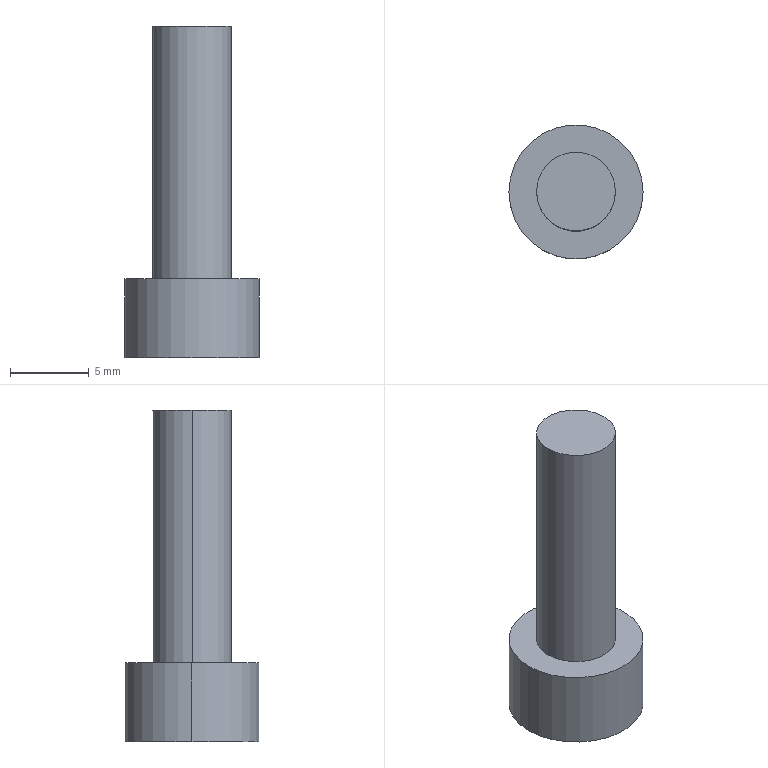Part | STEP file | LG M5_1.6F | 1 solid | 14 faces | box 8.5 x 8.5 x 21 mm | volume 562.896 mm3 | plane 10 | cylinder 4 | commonest cylinder face diameters 5 x2 8.5 x2
STEP:
#1=CARTESIAN_POINT('',(0.,0.,0.));
#2=DIRECTION('',(0.,0.,1.));
#3=DIRECTION('',(1.,0.,0.));
#4=AXIS2_PLACEMENT_3D('',#1,#2,#3);
#5=CARTESIAN_POINT('',(2.5,0.,16.));
#6=VERTEX_POINT('',#5);
#7=CARTESIAN_POINT('',(-2.5,0.,16.));
#8=VERTEX_POINT('',#7);
#9=CARTESIAN_POINT('',(0.,0.,16.));
#10=DIRECTION('',(0.,0.,1.));
#11=DIRECTION('',(1.,0.,0.));
#12=AXIS2_PLACEMENT_3D('',#9,#10,#11);
#13=CIRCLE('',#12,2.5);
#14=CARTESIAN_POINT('',(0.,0.,16.));
#15=DIRECTION('',(0.,0.,-1.));
#16=DIRECTION('',(-1.,0.,0.));
#17=AXIS2_PLACEMENT_3D('',#14,#15,#16);
#18=CYLINDRICAL_SURFACE('',#17,2.5);
#19=CARTESIAN_POINT('',(3.142,0.));
#20=DIRECTION('',(-1.,0.));
#21=VECTOR('',#20,1.);
#22=LINE('',#19,#21);
#23=(GEOMETRIC_REPRESENTATION_CONTEXT(2)PARAMETRIC_REPRESENTATION_CONTEXT()REPRESENTATION_CONTEXT('',''));
#24=DEFINITIONAL_REPRESENTATION('',(#22),#23);
#25=PCURVE('',#18,#24);
#26=CARTESIAN_POINT('',(0.,0.,16.));
#27=DIRECTION('',(0.,0.,1.));
#28=DIRECTION('',(1.,0.,0.));
#29=AXIS2_PLACEMENT_3D('',#26,#27,#28);
#30=PLANE('',#29);
#31=CARTESIAN_POINT('',(0.,0.));
#32=DIRECTION('',(1.,0.));
#33=AXIS2_PLACEMENT_2D('',#31,#32);
#34=CIRCLE('',#33,2.5);
#35=(GEOMETRIC_REPRESENTATION_CONTEXT(2)PARAMETRIC_REPRESENTATION_CONTEXT()REPRESENTATION_CONTEXT('',''));
#36=DEFINITIONAL_REPRESENTATION('',(#34),#35);
#37=PCURVE('',#30,#36);
#38=SURFACE_CURVE('',#13,(#25,#37),.PCURVE_S1.);
#39=EDGE_CURVE('',#6,#8,#38,.T.);
#40=ORIENTED_EDGE('',*,*,#39,.F.);
#41=CARTESIAN_POINT('',(2.5,0.,0.));
#42=VERTEX_POINT('',#41);
#43=CARTESIAN_POINT('',(2.5,0.,16.));
#44=DIRECTION('',(0.,0.,-1.));
#45=VECTOR('',#44,1.);
#46=LINE('',#43,#45);
#47=CARTESIAN_POINT('',(3.142,0.));
#48=DIRECTION('',(0.,1.));
#49=VECTOR('',#48,1.);
#50=LINE('',#47,#49);
#51=(GEOMETRIC_REPRESENTATION_CONTEXT(2)PARAMETRIC_REPRESENTATION_CONTEXT()REPRESENTATION_CONTEXT('',''));
#52=DEFINITIONAL_REPRESENTATION('',(#50),#51);
#53=PCURVE('',#18,#52);
#54=CARTESIAN_POINT('',(0.,0.,16.));
#55=DIRECTION('',(0.,0.,-1.));
#56=DIRECTION('',(-1.,0.,0.));
#57=AXIS2_PLACEMENT_3D('',#54,#55,#56);
#58=CYLINDRICAL_SURFACE('',#57,2.5);
#59=CARTESIAN_POINT('',(3.142,0.));
#60=DIRECTION('',(0.,1.));
#61=VECTOR('',#60,1.);
#62=LINE('',#59,#61);
#63=(GEOMETRIC_REPRESENTATION_CONTEXT(2)PARAMETRIC_REPRESENTATION_CONTEXT()REPRESENTATION_CONTEXT('',''));
#64=DEFINITIONAL_REPRESENTATION('',(#62),#63);
#65=PCURVE('',#58,#64);
#66=SURFACE_CURVE('',#46,(#53,#65),.PCURVE_S1.);
#67=EDGE_CURVE('',#6,#42,#66,.T.);
#68=ORIENTED_EDGE('',*,*,#67,.T.);
#69=CARTESIAN_POINT('',(-2.5,0.,0.));
#70=VERTEX_POINT('',#69);
#71=CARTESIAN_POINT('',(0.,0.,0.));
#72=DIRECTION('',(0.,0.,1.));
#73=DIRECTION('',(1.,0.,0.));
#74=AXIS2_PLACEMENT_3D('',#71,#72,#73);
#75=CIRCLE('',#74,2.5);
#76=CARTESIAN_POINT('',(3.142,16.));
#77=DIRECTION('',(-1.,0.));
#78=VECTOR('',#77,1.);
#79=LINE('',#76,#78);
#80=(GEOMETRIC_REPRESENTATION_CONTEXT(2)PARAMETRIC_REPRESENTATION_CONTEXT()REPRESENTATION_CONTEXT('',''));
#81=DEFINITIONAL_REPRESENTATION('',(#79),#80);
#82=PCURVE('',#18,#81);
#83=CARTESIAN_POINT('',(0.,0.,0.));
#84=DIRECTION('',(0.,0.,1.));
#85=DIRECTION('',(1.,0.,0.));
#86=AXIS2_PLACEMENT_3D('',#83,#84,#85);
#87=PLANE('',#86);
#88=CARTESIAN_POINT('',(0.,0.));
#89=DIRECTION('',(1.,0.));
#90=AXIS2_PLACEMENT_2D('',#88,#89);
#91=CIRCLE('',#90,2.5);
#92=(GEOMETRIC_REPRESENTATION_CONTEXT(2)PARAMETRIC_REPRESENTATION_CONTEXT()REPRESENTATION_CONTEXT('',''));
#93=DEFINITIONAL_REPRESENTATION('',(#91),#92);
#94=PCURVE('',#87,#93);
#95=SURFACE_CURVE('',#75,(#82,#94),.PCURVE_S1.);
#96=EDGE_CURVE('',#42,#70,#95,.T.);
#97=ORIENTED_EDGE('',*,*,#96,.T.);
#98=CARTESIAN_POINT('',(-2.5,0.,16.));
#99=DIRECTION('',(0.,0.,-1.));
#100=VECTOR('',#99,1.);
#101=LINE('',#98,#100);
#102=CARTESIAN_POINT('',(0.,0.));
#103=DIRECTION('',(0.,1.));
#104=VECTOR('',#103,1.);
#105=LINE('',#102,#104);
#106=(GEOMETRIC_REPRESENTATION_CONTEXT(2)PARAMETRIC_REPRESENTATION_CONTEXT()REPRESENTATION_CONTEXT('',''));
#107=DEFINITIONAL_REPRESENTATION('',(#105),#106);
#108=PCURVE('',#18,#107);
#109=CARTESIAN_POINT('',(6.283,0.));
#110=DIRECTION('',(0.,1.));
#111=VECTOR('',#110,1.);
#112=LINE('',#109,#111);
#113=(GEOMETRIC_REPRESENTATION_CONTEXT(2)PARAMETRIC_REPRESENTATION_CONTEXT()REPRESENTATION_CONTEXT('',''));
#114=DEFINITIONAL_REPRESENTATION('',(#112),#113);
#115=PCURVE('',#58,#114);
#116=SURFACE_CURVE('',#101,(#108,#115),.PCURVE_S1.);
#117=EDGE_CURVE('',#8,#70,#116,.T.);
#118=ORIENTED_EDGE('',*,*,#117,.F.);
#119=EDGE_LOOP('',(#40,#68,#97,#118));
#120=FACE_BOUND('',#119,.T.);
#121=ADVANCED_FACE('',(#120),#18,.T.);
#122=CARTESIAN_POINT('',(4.25,0.,-5.));
#123=VERTEX_POINT('',#122);
#124=CARTESIAN_POINT('',(-4.25,0.,-5.));
#125=VERTEX_POINT('',#124);
#126=CARTESIAN_POINT('',(0.,0.,-5.));
#127=DIRECTION('',(0.,0.,1.));
#128=DIRECTION('',(1.,0.,0.));
#129=AXIS2_PLACEMENT_3D('',#126,#127,#128);
#130=CIRCLE('',#129,4.25);
#131=CARTESIAN_POINT('',(0.,0.,-5.));
#132=DIRECTION('',(0.,0.,1.));
#133=DIRECTION('',(1.,0.,0.));
#134=AXIS2_PLACEMENT_3D('',#131,#132,#133);
#135=CYLINDRICAL_SURFACE('',#134,4.25);
#136=CARTESIAN_POINT('',(0.,0.));
#137=DIRECTION('',(1.,0.));
#138=VECTOR('',#137,1.);
#139=LINE('',#136,#138);
#140=(GEOMETRIC_REPRESENTATION_CONTEXT(2)PARAMETRIC_REPRESENTATION_CONTEXT()REPRESENTATION_CONTEXT('',''));
#141=DEFINITIONAL_REPRESENTATION('',(#139),#140);
#142=PCURVE('',#135,#141);
#143=CARTESIAN_POINT('',(0.,0.,-5.));
#144=DIRECTION('',(0.,0.,1.));
#145=DIRECTION('',(1.,0.,0.));
#146=AXIS2_PLACEMENT_3D('',#143,#144,#145);
#147=PLANE('',#146);
#148=CARTESIAN_POINT('',(0.,0.));
#149=DIRECTION('',(1.,0.));
#150=AXIS2_PLACEMENT_2D('',#148,#149);
#151=CIRCLE('',#150,4.25);
#152=(GEOMETRIC_REPRESENTATION_CONTEXT(2)PARAMETRIC_REPRESENTATION_CONTEXT()REPRESENTATION_CONTEXT('',''));
#153=DEFINITIONAL_REPRESENTATION('',(#151),#152);
#154=PCURVE('',#147,#153);
#155=SURFACE_CURVE('',#130,(#142,#154),.PCURVE_S1.);
#156=EDGE_CURVE('',#123,#125,#155,.T.);
#157=ORIENTED_EDGE('',*,*,#156,.T.);
#158=CARTESIAN_POINT('',(-4.25,0.,0.));
#159=VERTEX_POINT('',#158);
#160=CARTESIAN_POINT('',(-4.25,0.,-5.));
#161=DIRECTION('',(0.,0.,1.));
#162=VECTOR('',#161,1.);
#163=LINE('',#160,#162);
#164=CARTESIAN_POINT('',(3.142,0.));
#165=DIRECTION('',(0.,1.));
#166=VECTOR('',#165,1.);
#167=LINE('',#164,#166);
#168=(GEOMETRIC_REPRESENTATION_CONTEXT(2)PARAMETRIC_REPRESENTATION_CONTEXT()REPRESENTATION_CONTEXT('',''));
#169=DEFINITIONAL_REPRESENTATION('',(#167),#168);
#170=PCURVE('',#135,#169);
#171=CARTESIAN_POINT('',(0.,0.,-5.));
#172=DIRECTION('',(0.,0.,1.));
#173=DIRECTION('',(1.,0.,0.));
#174=AXIS2_PLACEMENT_3D('',#171,#172,#173);
#175=CYLINDRICAL_SURFACE('',#174,4.25);
#176=CARTESIAN_POINT('',(3.142,0.));
#177=DIRECTION('',(0.,1.));
#178=VECTOR('',#177,1.);
#179=LINE('',#176,#178);
#180=(GEOMETRIC_REPRESENTATION_CONTEXT(2)PARAMETRIC_REPRESENTATION_CONTEXT()REPRESENTATION_CONTEXT('',''));
#181=DEFINITIONAL_REPRESENTATION('',(#179),#180);
#182=PCURVE('',#175,#181);
#183=SURFACE_CURVE('',#163,(#170,#182),.PCURVE_S1.);
#184=EDGE_CURVE('',#125,#159,#183,.T.);
#185=ORIENTED_EDGE('',*,*,#184,.T.);
#186=CARTESIAN_POINT('',(4.25,0.,0.));
#187=VERTEX_POINT('',#186);
#188=CARTESIAN_POINT('',(0.,0.,0.));
#189=DIRECTION('',(0.,0.,1.));
#190=DIRECTION('',(1.,0.,0.));
#191=AXIS2_PLACEMENT_3D('',#188,#189,#190);
#192=CIRCLE('',#191,4.25);
#193=CARTESIAN_POINT('',(0.,5.));
#194=DIRECTION('',(1.,0.));
#195=VECTOR('',#194,1.);
#196=LINE('',#193,#195);
#197=(GEOMETRIC_REPRESENTATION_CONTEXT(2)PARAMETRIC_REPRESENTATION_CONTEXT()REPRESENTATION_CONTEXT('',''));
#198=DEFINITIONAL_REPRESENTATION('',(#196),#197);
#199=PCURVE('',#135,#198);
#200=CARTESIAN_POINT('',(0.,0.));
#201=DIRECTION('',(1.,0.));
#202=AXIS2_PLACEMENT_2D('',#200,#201);
#203=CIRCLE('',#202,4.25);
#204=(GEOMETRIC_REPRESENTATION_CONTEXT(2)PARAMETRIC_REPRESENTATION_CONTEXT()REPRESENTATION_CONTEXT('',''));
#205=DEFINITIONAL_REPRESENTATION('',(#203),#204);
#206=PCURVE('',#87,#205);
#207=SURFACE_CURVE('',#192,(#199,#206),.PCURVE_S1.);
#208=EDGE_CURVE('',#187,#159,#207,.T.);
#209=ORIENTED_EDGE('',*,*,#208,.F.);
#210=CARTESIAN_POINT('',(4.25,0.,-5.));
#211=DIRECTION('',(0.,0.,1.));
#212=VECTOR('',#211,1.);
#213=LINE('',#210,#212);
#214=CARTESIAN_POINT('',(0.,0.));
#215=DIRECTION('',(0.,1.));
#216=VECTOR('',#215,1.);
#217=LINE('',#214,#216);
#218=(GEOMETRIC_REPRESENTATION_CONTEXT(2)PARAMETRIC_REPRESENTATION_CONTEXT()REPRESENTATION_CONTEXT('',''));
#219=DEFINITIONAL_REPRESENTATION('',(#217),#218);
#220=PCURVE('',#135,#219);
#221=CARTESIAN_POINT('',(6.283,0.));
#222=DIRECTION('',(0.,1.));
#223=VECTOR('',#222,1.);
#224=LINE('',#221,#223);
#225=(GEOMETRIC_REPRESENTATION_CONTEXT(2)PARAMETRIC_REPRESENTATION_CONTEXT()REPRESENTATION_CONTEXT('',''));
#226=DEFINITIONAL_REPRESENTATION('',(#224),#225);
#227=PCURVE('',#175,#226);
#228=SURFACE_CURVE('',#213,(#220,#227),.PCURVE_S1.);
#229=EDGE_CURVE('',#123,#187,#228,.T.);
#230=ORIENTED_EDGE('',*,*,#229,.F.);
#231=EDGE_LOOP('',(#157,#185,#209,#230));
#232=FACE_BOUND('',#231,.T.);
#233=ADVANCED_FACE('',(#232),#135,.T.);
#234=ORIENTED_EDGE('',*,*,#208,.T.);
#235=CARTESIAN_POINT('',(0.,0.,0.));
#236=DIRECTION('',(0.,0.,1.));
#237=DIRECTION('',(1.,0.,0.));
#238=AXIS2_PLACEMENT_3D('',#235,#236,#237);
#239=CIRCLE('',#238,4.25);
#240=CARTESIAN_POINT('',(0.,0.));
#241=DIRECTION('',(1.,0.));
#242=AXIS2_PLACEMENT_2D('',#240,#241);
#243=CIRCLE('',#242,4.25);
#244=(GEOMETRIC_REPRESENTATION_CONTEXT(2)PARAMETRIC_REPRESENTATION_CONTEXT()REPRESENTATION_CONTEXT('',''));
#245=DEFINITIONAL_REPRESENTATION('',(#243),#244);
#246=PCURVE('',#87,#245);
#247=CARTESIAN_POINT('',(0.,5.));
#248=DIRECTION('',(1.,0.));
#249=VECTOR('',#248,1.);
#250=LINE('',#247,#249);
#251=(GEOMETRIC_REPRESENTATION_CONTEXT(2)PARAMETRIC_REPRESENTATION_CONTEXT()REPRESENTATION_CONTEXT('',''));
#252=DEFINITIONAL_REPRESENTATION('',(#250),#251);
#253=PCURVE('',#175,#252);
#254=SURFACE_CURVE('',#239,(#246,#253),.PCURVE_S1.);
#255=EDGE_CURVE('',#159,#187,#254,.T.);
#256=ORIENTED_EDGE('',*,*,#255,.T.);
#257=EDGE_LOOP('',(#234,#256));
#258=FACE_BOUND('',#257,.T.);
#259=CARTESIAN_POINT('',(0.,0.,0.));
#260=DIRECTION('',(0.,0.,1.));
#261=DIRECTION('',(1.,0.,0.));
#262=AXIS2_PLACEMENT_3D('',#259,#260,#261);
#263=CIRCLE('',#262,2.5);
#264=CARTESIAN_POINT('',(0.,0.));
#265=DIRECTION('',(1.,0.));
#266=AXIS2_PLACEMENT_2D('',#264,#265);
#267=CIRCLE('',#266,2.5);
#268=(GEOMETRIC_REPRESENTATION_CONTEXT(2)PARAMETRIC_REPRESENTATION_CONTEXT()REPRESENTATION_CONTEXT('',''));
#269=DEFINITIONAL_REPRESENTATION('',(#267),#268);
#270=PCURVE('',#87,#269);
#271=CARTESIAN_POINT('',(9.425,16.));
#272=DIRECTION('',(-1.,0.));
#273=VECTOR('',#272,1.);
#274=LINE('',#271,#273);
#275=(GEOMETRIC_REPRESENTATION_CONTEXT(2)PARAMETRIC_REPRESENTATION_CONTEXT()REPRESENTATION_CONTEXT('',''));
#276=DEFINITIONAL_REPRESENTATION('',(#274),#275);
#277=PCURVE('',#58,#276);
#278=SURFACE_CURVE('',#263,(#270,#277),.PCURVE_S1.);
#279=EDGE_CURVE('',#70,#42,#278,.T.);
#280=ORIENTED_EDGE('',*,*,#279,.F.);
#281=ORIENTED_EDGE('',*,*,#96,.F.);
#282=EDGE_LOOP('',(#280,#281));
#283=FACE_BOUND('',#282,.T.);
#284=ADVANCED_FACE('',(#258,#283),#87,.T.);
#285=ORIENTED_EDGE('',*,*,#184,.F.);
#286=CARTESIAN_POINT('',(0.,0.,-5.));
#287=DIRECTION('',(0.,0.,1.));
#288=DIRECTION('',(1.,0.,0.));
#289=AXIS2_PLACEMENT_3D('',#286,#287,#288);
#290=CIRCLE('',#289,4.25);
#291=CARTESIAN_POINT('',(0.,0.));
#292=DIRECTION('',(1.,0.));
#293=VECTOR('',#292,1.);
#294=LINE('',#291,#293);
#295=(GEOMETRIC_REPRESENTATION_CONTEXT(2)PARAMETRIC_REPRESENTATION_CONTEXT()REPRESENTATION_CONTEXT('',''));
#296=DEFINITIONAL_REPRESENTATION('',(#294),#295);
#297=PCURVE('',#175,#296);
#298=CARTESIAN_POINT('',(0.,0.));
#299=DIRECTION('',(1.,0.));
#300=AXIS2_PLACEMENT_2D('',#298,#299);
#301=CIRCLE('',#300,4.25);
#302=(GEOMETRIC_REPRESENTATION_CONTEXT(2)PARAMETRIC_REPRESENTATION_CONTEXT()REPRESENTATION_CONTEXT('',''));
#303=DEFINITIONAL_REPRESENTATION('',(#301),#302);
#304=PCURVE('',#147,#303);
#305=SURFACE_CURVE('',#290,(#297,#304),.PCURVE_S1.);
#306=EDGE_CURVE('',#125,#123,#305,.T.);
#307=ORIENTED_EDGE('',*,*,#306,.T.);
#308=ORIENTED_EDGE('',*,*,#229,.T.);
#309=ORIENTED_EDGE('',*,*,#255,.F.);
#310=EDGE_LOOP('',(#285,#307,#308,#309));
#311=FACE_BOUND('',#310,.T.);
#312=ADVANCED_FACE('',(#311),#175,.T.);
#313=CARTESIAN_POINT('',(-2.321,0.,-5.));
#314=VERTEX_POINT('',#313);
#315=CARTESIAN_POINT('',(-1.16,2.01,-5.));
#316=VERTEX_POINT('',#315);
#317=CARTESIAN_POINT('',(-2.321,0.,-5.));
#318=DIRECTION('',(0.5,0.866,0.));
#319=VECTOR('',#318,1.);
#320=LINE('',#317,#319);
#321=CARTESIAN_POINT('',(-2.321,0.));
#322=DIRECTION('',(0.5,0.866));
#323=VECTOR('',#322,1.);
#324=LINE('',#321,#323);
#325=(GEOMETRIC_REPRESENTATION_CONTEXT(2)PARAMETRIC_REPRESENTATION_CONTEXT()REPRESENTATION_CONTEXT('',''));
#326=DEFINITIONAL_REPRESENTATION('',(#324),#325);
#327=PCURVE('',#147,#326);
#328=CARTESIAN_POINT('',(-2.321,0.,-2.5));
#329=DIRECTION('',(-0.866,0.5,0.));
#330=DIRECTION('',(-0.5,-0.866,0.));
#331=AXIS2_PLACEMENT_3D('',#328,#329,#330);
#332=PLANE('',#331);
#333=CARTESIAN_POINT('',(0.,-2.5));
#334=DIRECTION('',(-1.,0.));
#335=VECTOR('',#334,1.);
#336=LINE('',#333,#335);
#337=(GEOMETRIC_REPRESENTATION_CONTEXT(2)PARAMETRIC_REPRESENTATION_CONTEXT()REPRESENTATION_CONTEXT('',''));
#338=DEFINITIONAL_REPRESENTATION('',(#336),#337);
#339=PCURVE('',#332,#338);
#340=SURFACE_CURVE('',#320,(#327,#339),.PCURVE_S1.);
#341=EDGE_CURVE('',#314,#316,#340,.T.);
#342=ORIENTED_EDGE('',*,*,#341,.F.);
#343=CARTESIAN_POINT('',(-1.16,-2.01,-5.));
#344=VERTEX_POINT('',#343);
#345=CARTESIAN_POINT('',(-1.16,-2.01,-5.));
#346=DIRECTION('',(-0.5,0.866,0.));
#347=VECTOR('',#346,1.);
#348=LINE('',#345,#347);
#349=CARTESIAN_POINT('',(-1.16,-2.01));
#350=DIRECTION('',(-0.5,0.866));
#351=VECTOR('',#350,1.);
#352=LINE('',#349,#351);
#353=(GEOMETRIC_REPRESENTATION_CONTEXT(2)PARAMETRIC_REPRESENTATION_CONTEXT()REPRESENTATION_CONTEXT('',''));
#354=DEFINITIONAL_REPRESENTATION('',(#352),#353);
#355=PCURVE('',#147,#354);
#356=CARTESIAN_POINT('',(-1.16,-2.01,-2.5));
#357=DIRECTION('',(-0.866,-0.5,0.));
#358=DIRECTION('',(0.5,-0.866,0.));
#359=AXIS2_PLACEMENT_3D('',#356,#357,#358);
#360=PLANE('',#359);
#361=CARTESIAN_POINT('',(0.,-2.5));
#362=DIRECTION('',(-1.,0.));
#363=VECTOR('',#362,1.);
#364=LINE('',#361,#363);
#365=(GEOMETRIC_REPRESENTATION_CONTEXT(2)PARAMETRIC_REPRESENTATION_CONTEXT()REPRESENTATION_CONTEXT('',''));
#366=DEFINITIONAL_REPRESENTATION('',(#364),#365);
#367=PCURVE('',#360,#366);
#368=SURFACE_CURVE('',#348,(#355,#367),.PCURVE_S1.);
#369=EDGE_CURVE('',#344,#314,#368,.T.);
#370=ORIENTED_EDGE('',*,*,#369,.F.);
#371=CARTESIAN_POINT('',(1.16,-2.01,-5.));
#372=VERTEX_POINT('',#371);
#373=CARTESIAN_POINT('',(1.16,-2.01,-5.));
#374=DIRECTION('',(-1.,0.,0.));
#375=VECTOR('',#374,1.);
#376=LINE('',#373,#375);
#377=CARTESIAN_POINT('',(1.16,-2.01));
#378=DIRECTION('',(-1.,0.));
#379=VECTOR('',#378,1.);
#380=LINE('',#377,#379);
#381=(GEOMETRIC_REPRESENTATION_CONTEXT(2)PARAMETRIC_REPRESENTATION_CONTEXT()REPRESENTATION_CONTEXT('',''));
#382=DEFINITIONAL_REPRESENTATION('',(#380),#381);
#383=PCURVE('',#147,#382);
#384=CARTESIAN_POINT('',(1.16,-2.01,-2.5));
#385=DIRECTION('',(0.,-1.,0.));
#386=DIRECTION('',(0.,0.,-1.));
#387=AXIS2_PLACEMENT_3D('',#384,#385,#386);
#388=PLANE('',#387);
#389=CARTESIAN_POINT('',(2.5,0.));
#390=DIRECTION('',(0.,-1.));
#391=VECTOR('',#390,1.);
#392=LINE('',#389,#391);
#393=(GEOMETRIC_REPRESENTATION_CONTEXT(2)PARAMETRIC_REPRESENTATION_CONTEXT()REPRESENTATION_CONTEXT('',''));
#394=DEFINITIONAL_REPRESENTATION('',(#392),#393);
#395=PCURVE('',#388,#394);
#396=SURFACE_CURVE('',#376,(#383,#395),.PCURVE_S1.);
#397=EDGE_CURVE('',#372,#344,#396,.T.);
#398=ORIENTED_EDGE('',*,*,#397,.F.);
#399=CARTESIAN_POINT('',(2.321,0.,-5.));
#400=VERTEX_POINT('',#399);
#401=CARTESIAN_POINT('',(2.321,0.,-5.));
#402=DIRECTION('',(-0.5,-0.866,0.));
#403=VECTOR('',#402,1.);
#404=LINE('',#401,#403);
#405=CARTESIAN_POINT('',(2.321,0.));
#406=DIRECTION('',(-0.5,-0.866));
#407=VECTOR('',#406,1.);
#408=LINE('',#405,#407);
#409=(GEOMETRIC_REPRESENTATION_CONTEXT(2)PARAMETRIC_REPRESENTATION_CONTEXT()REPRESENTATION_CONTEXT('',''));
#410=DEFINITIONAL_REPRESENTATION('',(#408),#409);
#411=PCURVE('',#147,#410);
#412=CARTESIAN_POINT('',(2.321,0.,-2.5));
#413=DIRECTION('',(0.866,-0.5,0.));
#414=DIRECTION('',(0.5,0.866,0.));
#415=AXIS2_PLACEMENT_3D('',#412,#413,#414);
#416=PLANE('',#415);
#417=CARTESIAN_POINT('',(0.,-2.5));
#418=DIRECTION('',(-1.,0.));
#419=VECTOR('',#418,1.);
#420=LINE('',#417,#419);
#421=(GEOMETRIC_REPRESENTATION_CONTEXT(2)PARAMETRIC_REPRESENTATION_CONTEXT()REPRESENTATION_CONTEXT('',''));
#422=DEFINITIONAL_REPRESENTATION('',(#420),#421);
#423=PCURVE('',#416,#422);
#424=SURFACE_CURVE('',#404,(#411,#423),.PCURVE_S1.);
#425=EDGE_CURVE('',#400,#372,#424,.T.);
#426=ORIENTED_EDGE('',*,*,#425,.F.);
#427=CARTESIAN_POINT('',(1.16,2.01,-5.));
#428=VERTEX_POINT('',#427);
#429=CARTESIAN_POINT('',(1.16,2.01,-5.));
#430=DIRECTION('',(0.5,-0.866,0.));
#431=VECTOR('',#430,1.);
#432=LINE('',#429,#431);
#433=CARTESIAN_POINT('',(1.16,2.01));
#434=DIRECTION('',(0.5,-0.866));
#435=VECTOR('',#434,1.);
#436=LINE('',#433,#435);
#437=(GEOMETRIC_REPRESENTATION_CONTEXT(2)PARAMETRIC_REPRESENTATION_CONTEXT()REPRESENTATION_CONTEXT('',''));
#438=DEFINITIONAL_REPRESENTATION('',(#436),#437);
#439=PCURVE('',#147,#438);
#440=CARTESIAN_POINT('',(1.16,2.01,-2.5));
#441=DIRECTION('',(0.866,0.5,0.));
#442=DIRECTION('',(-0.5,0.866,0.));
#443=AXIS2_PLACEMENT_3D('',#440,#441,#442);
#444=PLANE('',#443);
#445=CARTESIAN_POINT('',(0.,-2.5));
#446=DIRECTION('',(-1.,0.));
#447=VECTOR('',#446,1.);
#448=LINE('',#445,#447);
#449=(GEOMETRIC_REPRESENTATION_CONTEXT(2)PARAMETRIC_REPRESENTATION_CONTEXT()REPRESENTATION_CONTEXT('',''));
#450=DEFINITIONAL_REPRESENTATION('',(#448),#449);
#451=PCURVE('',#444,#450);
#452=SURFACE_CURVE('',#432,(#439,#451),.PCURVE_S1.);
#453=EDGE_CURVE('',#428,#400,#452,.T.);
#454=ORIENTED_EDGE('',*,*,#453,.F.);
#455=CARTESIAN_POINT('',(-1.16,2.01,-5.));
#456=DIRECTION('',(1.,0.,0.));
#457=VECTOR('',#456,1.);
#458=LINE('',#455,#457);
#459=CARTESIAN_POINT('',(-1.16,2.01));
#460=DIRECTION('',(1.,0.));
#461=VECTOR('',#460,1.);
#462=LINE('',#459,#461);
#463=(GEOMETRIC_REPRESENTATION_CONTEXT(2)PARAMETRIC_REPRESENTATION_CONTEXT()REPRESENTATION_CONTEXT('',''));
#464=DEFINITIONAL_REPRESENTATION('',(#462),#463);
#465=PCURVE('',#147,#464);
#466=CARTESIAN_POINT('',(-1.16,2.01,-2.5));
#467=DIRECTION('',(0.,1.,0.));
#468=DIRECTION('',(0.,0.,1.));
#469=AXIS2_PLACEMENT_3D('',#466,#467,#468);
#470=PLANE('',#469);
#471=CARTESIAN_POINT('',(-2.5,0.));
#472=DIRECTION('',(0.,1.));
#473=VECTOR('',#472,1.);
#474=LINE('',#471,#473);
#475=(GEOMETRIC_REPRESENTATION_CONTEXT(2)PARAMETRIC_REPRESENTATION_CONTEXT()REPRESENTATION_CONTEXT('',''));
#476=DEFINITIONAL_REPRESENTATION('',(#474),#475);
#477=PCURVE('',#470,#476);
#478=SURFACE_CURVE('',#458,(#465,#477),.PCURVE_S1.);
#479=EDGE_CURVE('',#316,#428,#478,.T.);
#480=ORIENTED_EDGE('',*,*,#479,.F.);
#481=EDGE_LOOP('',(#342,#370,#398,#426,#454,#480));
#482=FACE_BOUND('',#481,.T.);
#483=ORIENTED_EDGE('',*,*,#156,.F.);
#484=ORIENTED_EDGE('',*,*,#306,.F.);
#485=EDGE_LOOP('',(#483,#484));
#486=FACE_BOUND('',#485,.T.);
#487=ADVANCED_FACE('',(#482,#486),#147,.F.);
#488=ORIENTED_EDGE('',*,*,#67,.F.);
#489=CARTESIAN_POINT('',(0.,0.,16.));
#490=DIRECTION('',(0.,0.,1.));
#491=DIRECTION('',(1.,0.,0.));
#492=AXIS2_PLACEMENT_3D('',#489,#490,#491);
#493=CIRCLE('',#492,2.5);
#494=CARTESIAN_POINT('',(9.425,0.));
#495=DIRECTION('',(-1.,0.));
#496=VECTOR('',#495,1.);
#497=LINE('',#494,#496);
#498=(GEOMETRIC_REPRESENTATION_CONTEXT(2)PARAMETRIC_REPRESENTATION_CONTEXT()REPRESENTATION_CONTEXT('',''));
#499=DEFINITIONAL_REPRESENTATION('',(#497),#498);
#500=PCURVE('',#58,#499);
#501=CARTESIAN_POINT('',(0.,0.));
#502=DIRECTION('',(1.,0.));
#503=AXIS2_PLACEMENT_2D('',#501,#502);
#504=CIRCLE('',#503,2.5);
#505=(GEOMETRIC_REPRESENTATION_CONTEXT(2)PARAMETRIC_REPRESENTATION_CONTEXT()REPRESENTATION_CONTEXT('',''));
#506=DEFINITIONAL_REPRESENTATION('',(#504),#505);
#507=PCURVE('',#30,#506);
#508=SURFACE_CURVE('',#493,(#500,#507),.PCURVE_S1.);
#509=EDGE_CURVE('',#8,#6,#508,.T.);
#510=ORIENTED_EDGE('',*,*,#509,.F.);
#511=ORIENTED_EDGE('',*,*,#117,.T.);
#512=ORIENTED_EDGE('',*,*,#279,.T.);
#513=EDGE_LOOP('',(#488,#510,#511,#512));
#514=FACE_BOUND('',#513,.T.);
#515=ADVANCED_FACE('',(#514),#58,.T.);
#516=ORIENTED_EDGE('',*,*,#509,.T.);
#517=ORIENTED_EDGE('',*,*,#39,.T.);
#518=EDGE_LOOP('',(#516,#517));
#519=FACE_BOUND('',#518,.T.);
#520=ADVANCED_FACE('',(#519),#30,.T.);
#521=ORIENTED_EDGE('',*,*,#369,.T.);
#522=CARTESIAN_POINT('',(-2.321,0.,-2.5));
#523=VERTEX_POINT('',#522);
#524=CARTESIAN_POINT('',(-2.321,0.,-2.5));
#525=DIRECTION('',(0.,0.,-1.));
#526=VECTOR('',#525,1.);
#527=LINE('',#524,#526);
#528=CARTESIAN_POINT('',(-2.321,0.));
#529=DIRECTION('',(0.,-1.));
#530=VECTOR('',#529,1.);
#531=LINE('',#528,#530);
#532=(GEOMETRIC_REPRESENTATION_CONTEXT(2)PARAMETRIC_REPRESENTATION_CONTEXT()REPRESENTATION_CONTEXT('',''));
#533=DEFINITIONAL_REPRESENTATION('',(#531),#532);
#534=PCURVE('',#360,#533);
#535=CARTESIAN_POINT('',(0.,0.));
#536=DIRECTION('',(0.,-1.));
#537=VECTOR('',#536,1.);
#538=LINE('',#535,#537);
#539=(GEOMETRIC_REPRESENTATION_CONTEXT(2)PARAMETRIC_REPRESENTATION_CONTEXT()REPRESENTATION_CONTEXT('',''));
#540=DEFINITIONAL_REPRESENTATION('',(#538),#539);
#541=PCURVE('',#332,#540);
#542=SURFACE_CURVE('',#527,(#534,#541),.PCURVE_S1.);
#543=EDGE_CURVE('',#523,#314,#542,.T.);
#544=ORIENTED_EDGE('',*,*,#543,.F.);
#545=CARTESIAN_POINT('',(-1.16,-2.01,-2.5));
#546=VERTEX_POINT('',#545);
#547=CARTESIAN_POINT('',(-1.16,-2.01,-2.5));
#548=DIRECTION('',(-0.5,0.866,0.));
#549=VECTOR('',#548,1.);
#550=LINE('',#547,#549);
#551=CARTESIAN_POINT('',(0.,0.));
#552=DIRECTION('',(-1.,0.));
#553=VECTOR('',#552,1.);
#554=LINE('',#551,#553);
#555=(GEOMETRIC_REPRESENTATION_CONTEXT(2)PARAMETRIC_REPRESENTATION_CONTEXT()REPRESENTATION_CONTEXT('',''));
#556=DEFINITIONAL_REPRESENTATION('',(#554),#555);
#557=PCURVE('',#360,#556);
#558=CARTESIAN_POINT('',(0.,0.,-2.5));
#559=DIRECTION('',(0.,0.,-1.));
#560=DIRECTION('',(-1.,0.,0.));
#561=AXIS2_PLACEMENT_3D('',#558,#559,#560);
#562=PLANE('',#561);
#563=CARTESIAN_POINT('',(1.16,-2.01));
#564=DIRECTION('',(0.5,0.866));
#565=VECTOR('',#564,1.);
#566=LINE('',#563,#565);
#567=(GEOMETRIC_REPRESENTATION_CONTEXT(2)PARAMETRIC_REPRESENTATION_CONTEXT()REPRESENTATION_CONTEXT('',''));
#568=DEFINITIONAL_REPRESENTATION('',(#566),#567);
#569=PCURVE('',#562,#568);
#570=SURFACE_CURVE('',#550,(#557,#569),.PCURVE_S1.);
#571=EDGE_CURVE('',#546,#523,#570,.T.);
#572=ORIENTED_EDGE('',*,*,#571,.F.);
#573=CARTESIAN_POINT('',(-1.16,-2.01,-2.5));
#574=DIRECTION('',(0.,0.,-1.));
#575=VECTOR('',#574,1.);
#576=LINE('',#573,#575);
#577=CARTESIAN_POINT('',(0.,0.));
#578=DIRECTION('',(0.,-1.));
#579=VECTOR('',#578,1.);
#580=LINE('',#577,#579);
#581=(GEOMETRIC_REPRESENTATION_CONTEXT(2)PARAMETRIC_REPRESENTATION_CONTEXT()REPRESENTATION_CONTEXT('',''));
#582=DEFINITIONAL_REPRESENTATION('',(#580),#581);
#583=PCURVE('',#360,#582);
#584=CARTESIAN_POINT('',(0.,-2.321));
#585=DIRECTION('',(1.,0.));
#586=VECTOR('',#585,1.);
#587=LINE('',#584,#586);
#588=(GEOMETRIC_REPRESENTATION_CONTEXT(2)PARAMETRIC_REPRESENTATION_CONTEXT()REPRESENTATION_CONTEXT('',''));
#589=DEFINITIONAL_REPRESENTATION('',(#587),#588);
#590=PCURVE('',#388,#589);
#591=SURFACE_CURVE('',#576,(#583,#590),.PCURVE_S1.);
#592=EDGE_CURVE('',#546,#344,#591,.T.);
#593=ORIENTED_EDGE('',*,*,#592,.T.);
#594=EDGE_LOOP('',(#521,#544,#572,#593));
#595=FACE_BOUND('',#594,.T.);
#596=ADVANCED_FACE('',(#595),#360,.F.);
#597=ORIENTED_EDGE('',*,*,#397,.T.);
#598=ORIENTED_EDGE('',*,*,#592,.F.);
#599=CARTESIAN_POINT('',(1.16,-2.01,-2.5));
#600=VERTEX_POINT('',#599);
#601=CARTESIAN_POINT('',(1.16,-2.01,-2.5));
#602=DIRECTION('',(-1.,0.,0.));
#603=VECTOR('',#602,1.);
#604=LINE('',#601,#603);
#605=CARTESIAN_POINT('',(0.,0.));
#606=DIRECTION('',(0.,-1.));
#607=VECTOR('',#606,1.);
#608=LINE('',#605,#607);
#609=(GEOMETRIC_REPRESENTATION_CONTEXT(2)PARAMETRIC_REPRESENTATION_CONTEXT()REPRESENTATION_CONTEXT('',''));
#610=DEFINITIONAL_REPRESENTATION('',(#608),#609);
#611=PCURVE('',#388,#610);
#612=CARTESIAN_POINT('',(-1.16,-2.01));
#613=DIRECTION('',(1.,0.));
#614=VECTOR('',#613,1.);
#615=LINE('',#612,#614);
#616=(GEOMETRIC_REPRESENTATION_CONTEXT(2)PARAMETRIC_REPRESENTATION_CONTEXT()REPRESENTATION_CONTEXT('',''));
#617=DEFINITIONAL_REPRESENTATION('',(#615),#616);
#618=PCURVE('',#562,#617);
#619=SURFACE_CURVE('',#604,(#611,#618),.PCURVE_S1.);
#620=EDGE_CURVE('',#600,#546,#619,.T.);
#621=ORIENTED_EDGE('',*,*,#620,.F.);
#622=CARTESIAN_POINT('',(1.16,-2.01,-2.5));
#623=DIRECTION('',(0.,0.,-1.));
#624=VECTOR('',#623,1.);
#625=LINE('',#622,#624);
#626=CARTESIAN_POINT('',(0.,0.));
#627=DIRECTION('',(1.,0.));
#628=VECTOR('',#627,1.);
#629=LINE('',#626,#628);
#630=(GEOMETRIC_REPRESENTATION_CONTEXT(2)PARAMETRIC_REPRESENTATION_CONTEXT()REPRESENTATION_CONTEXT('',''));
#631=DEFINITIONAL_REPRESENTATION('',(#629),#630);
#632=PCURVE('',#388,#631);
#633=CARTESIAN_POINT('',(-2.321,0.));
#634=DIRECTION('',(0.,-1.));
#635=VECTOR('',#634,1.);
#636=LINE('',#633,#635);
#637=(GEOMETRIC_REPRESENTATION_CONTEXT(2)PARAMETRIC_REPRESENTATION_CONTEXT()REPRESENTATION_CONTEXT('',''));
#638=DEFINITIONAL_REPRESENTATION('',(#636),#637);
#639=PCURVE('',#416,#638);
#640=SURFACE_CURVE('',#625,(#632,#639),.PCURVE_S1.);
#641=EDGE_CURVE('',#600,#372,#640,.T.);
#642=ORIENTED_EDGE('',*,*,#641,.T.);
#643=EDGE_LOOP('',(#597,#598,#621,#642));
#644=FACE_BOUND('',#643,.T.);
#645=ADVANCED_FACE('',(#644),#388,.F.);
#646=ORIENTED_EDGE('',*,*,#425,.T.);
#647=ORIENTED_EDGE('',*,*,#641,.F.);
#648=CARTESIAN_POINT('',(2.321,0.,-2.5));
#649=VERTEX_POINT('',#648);
#650=CARTESIAN_POINT('',(2.321,0.,-2.5));
#651=DIRECTION('',(-0.5,-0.866,0.));
#652=VECTOR('',#651,1.);
#653=LINE('',#650,#652);
#654=CARTESIAN_POINT('',(0.,0.));
#655=DIRECTION('',(-1.,0.));
#656=VECTOR('',#655,1.);
#657=LINE('',#654,#656);
#658=(GEOMETRIC_REPRESENTATION_CONTEXT(2)PARAMETRIC_REPRESENTATION_CONTEXT()REPRESENTATION_CONTEXT('',''));
#659=DEFINITIONAL_REPRESENTATION('',(#657),#658);
#660=PCURVE('',#416,#659);
#661=CARTESIAN_POINT('',(-2.321,0.));
#662=DIRECTION('',(0.5,-0.866));
#663=VECTOR('',#662,1.);
#664=LINE('',#661,#663);
#665=(GEOMETRIC_REPRESENTATION_CONTEXT(2)PARAMETRIC_REPRESENTATION_CONTEXT()REPRESENTATION_CONTEXT('',''));
#666=DEFINITIONAL_REPRESENTATION('',(#664),#665);
#667=PCURVE('',#562,#666);
#668=SURFACE_CURVE('',#653,(#660,#667),.PCURVE_S1.);
#669=EDGE_CURVE('',#649,#600,#668,.T.);
#670=ORIENTED_EDGE('',*,*,#669,.F.);
#671=CARTESIAN_POINT('',(2.321,0.,-2.5));
#672=DIRECTION('',(0.,0.,-1.));
#673=VECTOR('',#672,1.);
#674=LINE('',#671,#673);
#675=CARTESIAN_POINT('',(0.,0.));
#676=DIRECTION('',(0.,-1.));
#677=VECTOR('',#676,1.);
#678=LINE('',#675,#677);
#679=(GEOMETRIC_REPRESENTATION_CONTEXT(2)PARAMETRIC_REPRESENTATION_CONTEXT()REPRESENTATION_CONTEXT('',''));
#680=DEFINITIONAL_REPRESENTATION('',(#678),#679);
#681=PCURVE('',#416,#680);
#682=CARTESIAN_POINT('',(-2.321,0.));
#683=DIRECTION('',(0.,-1.));
#684=VECTOR('',#683,1.);
#685=LINE('',#682,#684);
#686=(GEOMETRIC_REPRESENTATION_CONTEXT(2)PARAMETRIC_REPRESENTATION_CONTEXT()REPRESENTATION_CONTEXT('',''));
#687=DEFINITIONAL_REPRESENTATION('',(#685),#686);
#688=PCURVE('',#444,#687);
#689=SURFACE_CURVE('',#674,(#681,#688),.PCURVE_S1.);
#690=EDGE_CURVE('',#649,#400,#689,.T.);
#691=ORIENTED_EDGE('',*,*,#690,.T.);
#692=EDGE_LOOP('',(#646,#647,#670,#691));
#693=FACE_BOUND('',#692,.T.);
#694=ADVANCED_FACE('',(#693),#416,.F.);
#695=ORIENTED_EDGE('',*,*,#453,.T.);
#696=ORIENTED_EDGE('',*,*,#690,.F.);
#697=CARTESIAN_POINT('',(1.16,2.01,-2.5));
#698=VERTEX_POINT('',#697);
#699=CARTESIAN_POINT('',(1.16,2.01,-2.5));
#700=DIRECTION('',(0.5,-0.866,0.));
#701=VECTOR('',#700,1.);
#702=LINE('',#699,#701);
#703=CARTESIAN_POINT('',(0.,0.));
#704=DIRECTION('',(-1.,0.));
#705=VECTOR('',#704,1.);
#706=LINE('',#703,#705);
#707=(GEOMETRIC_REPRESENTATION_CONTEXT(2)PARAMETRIC_REPRESENTATION_CONTEXT()REPRESENTATION_CONTEXT('',''));
#708=DEFINITIONAL_REPRESENTATION('',(#706),#707);
#709=PCURVE('',#444,#708);
#710=CARTESIAN_POINT('',(-1.16,2.01));
#711=DIRECTION('',(-0.5,-0.866));
#712=VECTOR('',#711,1.);
#713=LINE('',#710,#712);
#714=(GEOMETRIC_REPRESENTATION_CONTEXT(2)PARAMETRIC_REPRESENTATION_CONTEXT()REPRESENTATION_CONTEXT('',''));
#715=DEFINITIONAL_REPRESENTATION('',(#713),#714);
#716=PCURVE('',#562,#715);
#717=SURFACE_CURVE('',#702,(#709,#716),.PCURVE_S1.);
#718=EDGE_CURVE('',#698,#649,#717,.T.);
#719=ORIENTED_EDGE('',*,*,#718,.F.);
#720=CARTESIAN_POINT('',(1.16,2.01,-2.5));
#721=DIRECTION('',(0.,0.,-1.));
#722=VECTOR('',#721,1.);
#723=LINE('',#720,#722);
#724=CARTESIAN_POINT('',(0.,0.));
#725=DIRECTION('',(0.,-1.));
#726=VECTOR('',#725,1.);
#727=LINE('',#724,#726);
#728=(GEOMETRIC_REPRESENTATION_CONTEXT(2)PARAMETRIC_REPRESENTATION_CONTEXT()REPRESENTATION_CONTEXT('',''));
#729=DEFINITIONAL_REPRESENTATION('',(#727),#728);
#730=PCURVE('',#444,#729);
#731=CARTESIAN_POINT('',(0.,2.321));
#732=DIRECTION('',(-1.,0.));
#733=VECTOR('',#732,1.);
#734=LINE('',#731,#733);
#735=(GEOMETRIC_REPRESENTATION_CONTEXT(2)PARAMETRIC_REPRESENTATION_CONTEXT()REPRESENTATION_CONTEXT('',''));
#736=DEFINITIONAL_REPRESENTATION('',(#734),#735);
#737=PCURVE('',#470,#736);
#738=SURFACE_CURVE('',#723,(#730,#737),.PCURVE_S1.);
#739=EDGE_CURVE('',#698,#428,#738,.T.);
#740=ORIENTED_EDGE('',*,*,#739,.T.);
#741=EDGE_LOOP('',(#695,#696,#719,#740));
#742=FACE_BOUND('',#741,.T.);
#743=ADVANCED_FACE('',(#742),#444,.F.);
#744=ORIENTED_EDGE('',*,*,#479,.T.);
#745=ORIENTED_EDGE('',*,*,#739,.F.);
#746=CARTESIAN_POINT('',(-1.16,2.01,-2.5));
#747=VERTEX_POINT('',#746);
#748=CARTESIAN_POINT('',(-1.16,2.01,-2.5));
#749=DIRECTION('',(1.,0.,0.));
#750=VECTOR('',#749,1.);
#751=LINE('',#748,#750);
#752=CARTESIAN_POINT('',(0.,0.));
#753=DIRECTION('',(0.,1.));
#754=VECTOR('',#753,1.);
#755=LINE('',#752,#754);
#756=(GEOMETRIC_REPRESENTATION_CONTEXT(2)PARAMETRIC_REPRESENTATION_CONTEXT()REPRESENTATION_CONTEXT('',''));
#757=DEFINITIONAL_REPRESENTATION('',(#755),#756);
#758=PCURVE('',#470,#757);
#759=CARTESIAN_POINT('',(1.16,2.01));
#760=DIRECTION('',(-1.,0.));
#761=VECTOR('',#760,1.);
#762=LINE('',#759,#761);
#763=(GEOMETRIC_REPRESENTATION_CONTEXT(2)PARAMETRIC_REPRESENTATION_CONTEXT()REPRESENTATION_CONTEXT('',''));
#764=DEFINITIONAL_REPRESENTATION('',(#762),#763);
#765=PCURVE('',#562,#764);
#766=SURFACE_CURVE('',#751,(#758,#765),.PCURVE_S1.);
#767=EDGE_CURVE('',#747,#698,#766,.T.);
#768=ORIENTED_EDGE('',*,*,#767,.F.);
#769=CARTESIAN_POINT('',(-1.16,2.01,-2.5));
#770=DIRECTION('',(0.,0.,-1.));
#771=VECTOR('',#770,1.);
#772=LINE('',#769,#771);
#773=CARTESIAN_POINT('',(0.,0.));
#774=DIRECTION('',(-1.,0.));
#775=VECTOR('',#774,1.);
#776=LINE('',#773,#775);
#777=(GEOMETRIC_REPRESENTATION_CONTEXT(2)PARAMETRIC_REPRESENTATION_CONTEXT()REPRESENTATION_CONTEXT('',''));
#778=DEFINITIONAL_REPRESENTATION('',(#776),#777);
#779=PCURVE('',#470,#778);
#780=CARTESIAN_POINT('',(-2.321,0.));
#781=DIRECTION('',(0.,-1.));
#782=VECTOR('',#781,1.);
#783=LINE('',#780,#782);
#784=(GEOMETRIC_REPRESENTATION_CONTEXT(2)PARAMETRIC_REPRESENTATION_CONTEXT()REPRESENTATION_CONTEXT('',''));
#785=DEFINITIONAL_REPRESENTATION('',(#783),#784);
#786=PCURVE('',#332,#785);
#787=SURFACE_CURVE('',#772,(#779,#786),.PCURVE_S1.);
#788=EDGE_CURVE('',#747,#316,#787,.T.);
#789=ORIENTED_EDGE('',*,*,#788,.T.);
#790=EDGE_LOOP('',(#744,#745,#768,#789));
#791=FACE_BOUND('',#790,.T.);
#792=ADVANCED_FACE('',(#791),#470,.F.);
#793=ORIENTED_EDGE('',*,*,#341,.T.);
#794=ORIENTED_EDGE('',*,*,#788,.F.);
#795=CARTESIAN_POINT('',(-2.321,0.,-2.5));
#796=DIRECTION('',(0.5,0.866,0.));
#797=VECTOR('',#796,1.);
#798=LINE('',#795,#797);
#799=CARTESIAN_POINT('',(0.,0.));
#800=DIRECTION('',(-1.,0.));
#801=VECTOR('',#800,1.);
#802=LINE('',#799,#801);
#803=(GEOMETRIC_REPRESENTATION_CONTEXT(2)PARAMETRIC_REPRESENTATION_CONTEXT()REPRESENTATION_CONTEXT('',''));
#804=DEFINITIONAL_REPRESENTATION('',(#802),#803);
#805=PCURVE('',#332,#804);
#806=CARTESIAN_POINT('',(2.321,0.));
#807=DIRECTION('',(-0.5,0.866));
#808=VECTOR('',#807,1.);
#809=LINE('',#806,#808);
#810=(GEOMETRIC_REPRESENTATION_CONTEXT(2)PARAMETRIC_REPRESENTATION_CONTEXT()REPRESENTATION_CONTEXT('',''));
#811=DEFINITIONAL_REPRESENTATION('',(#809),#810);
#812=PCURVE('',#562,#811);
#813=SURFACE_CURVE('',#798,(#805,#812),.PCURVE_S1.);
#814=EDGE_CURVE('',#523,#747,#813,.T.);
#815=ORIENTED_EDGE('',*,*,#814,.F.);
#816=ORIENTED_EDGE('',*,*,#543,.T.);
#817=EDGE_LOOP('',(#793,#794,#815,#816));
#818=FACE_BOUND('',#817,.T.);
#819=ADVANCED_FACE('',(#818),#332,.F.);
#820=ORIENTED_EDGE('',*,*,#571,.T.);
#821=ORIENTED_EDGE('',*,*,#814,.T.);
#822=ORIENTED_EDGE('',*,*,#767,.T.);
#823=ORIENTED_EDGE('',*,*,#718,.T.);
#824=ORIENTED_EDGE('',*,*,#669,.T.);
#825=ORIENTED_EDGE('',*,*,#620,.T.);
#826=EDGE_LOOP('',(#820,#821,#822,#823,#824,#825));
#827=FACE_BOUND('',#826,.T.);
#828=ADVANCED_FACE('',(#827),#562,.T.);
#829=CLOSED_SHELL('',(#121,#233,#284,#312,#487,#515,#520,#596,#645,#694,#743,#792,#819,#828));
#830=MANIFOLD_SOLID_BREP('',#829);
#831=(LENGTH_UNIT()NAMED_UNIT(*)SI_UNIT(.MILLI.,.METRE.));
#832=UNCERTAINTY_MEASURE_WITH_UNIT(LENGTH_MEASURE(0.0000001),#831,'','');
#833=(NAMED_UNIT(*)PLANE_ANGLE_UNIT()SI_UNIT($,.RADIAN.));
#834=(NAMED_UNIT(*)SI_UNIT($,.STERADIAN.)SOLID_ANGLE_UNIT());
#835=(GEOMETRIC_REPRESENTATION_CONTEXT(3)GLOBAL_UNCERTAINTY_ASSIGNED_CONTEXT((#832))GLOBAL_UNIT_ASSIGNED_CONTEXT((#831,#833,#834))REPRESENTATION_CONTEXT('',''));
#836=ADVANCED_BREP_SHAPE_REPRESENTATION('',(#4,#830),#835);